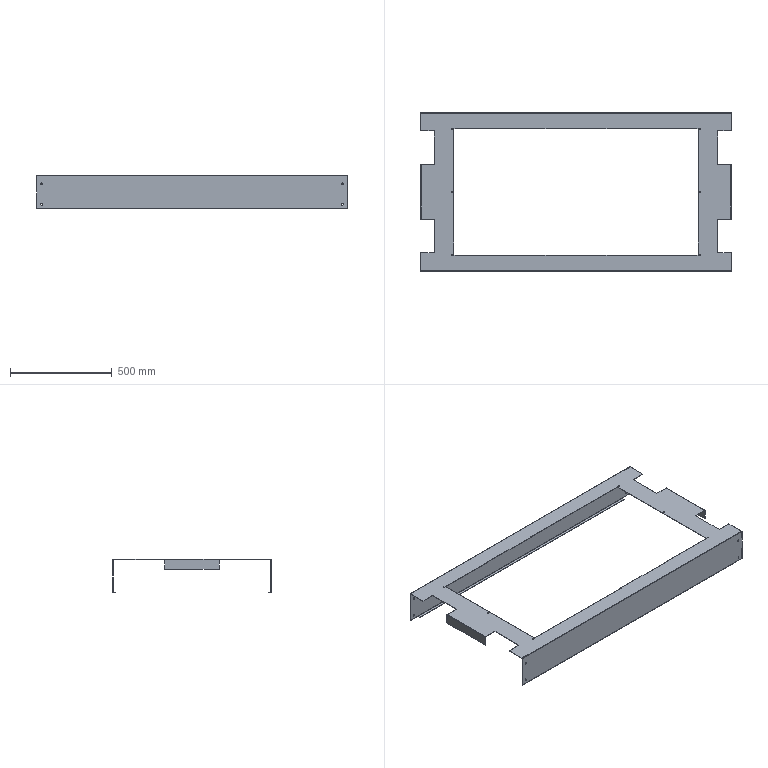Part | SolidWorks | features BaseBody 1 | 1 solid | 130 faces | box 1528 x 781 x 165 mm | volume 1922839 mm3 | plane 76 | cylinder 54 | commonest cylinder face diameters 5.5 x42 0.4 x6 4.4 x6